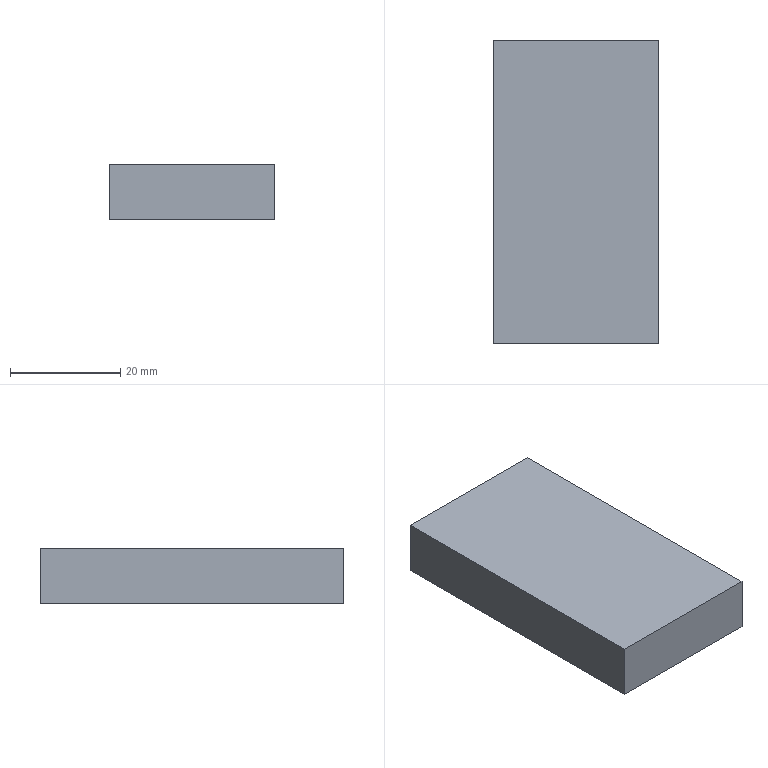Part | NX | features solid 2 | 1 solid | 6 faces | box 30 x 55 x 10 mm | volume 16500 mm3 | plane 6
STEP:
#1=CARTESIAN_POINT('',(660.,90.,-75.));
#2=VERTEX_POINT('',#1);
#3=CARTESIAN_POINT('',(660.,145.,-75.));
#4=VERTEX_POINT('',#3);
#5=CARTESIAN_POINT('',(660.,225.,-75.));
#6=DIRECTION('',(0.,-1.,0.));
#7=VECTOR('',#6,1000.);
#8=LINE('',#5,#7);
#9=EDGE_CURVE('',#2,#4,#8,.F.);
#10=ORIENTED_EDGE('',*,*,#9,.T.);
#11=CARTESIAN_POINT('',(660.,145.,-65.));
#12=VERTEX_POINT('',#11);
#13=CARTESIAN_POINT('',(660.,145.,-75.));
#14=DIRECTION('',(0.,0.,1.));
#15=VECTOR('',#14,1000.);
#16=LINE('',#13,#15);
#17=EDGE_CURVE('',#4,#12,#16,.T.);
#18=ORIENTED_EDGE('',*,*,#17,.T.);
#19=CARTESIAN_POINT('',(660.,90.,-65.));
#20=VERTEX_POINT('',#19);
#21=CARTESIAN_POINT('',(660.,225.,-65.));
#22=DIRECTION('',(0.,1.,0.));
#23=VECTOR('',#22,1000.);
#24=LINE('',#21,#23);
#25=EDGE_CURVE('',#20,#12,#24,.T.);
#26=ORIENTED_EDGE('',*,*,#25,.F.);
#27=CARTESIAN_POINT('',(660.,90.,-75.));
#28=DIRECTION('',(0.,0.,-1.));
#29=VECTOR('',#28,1000.);
#30=LINE('',#27,#29);
#31=EDGE_CURVE('',#20,#2,#30,.T.);
#32=ORIENTED_EDGE('',*,*,#31,.T.);
#33=EDGE_LOOP('',(#10,#18,#26,#32));
#34=FACE_BOUND('',#33,.T.);
#35=CARTESIAN_POINT('',(660.,225.,-75.));
#36=DIRECTION('',(1.,0.,0.));
#37=DIRECTION('',(0.,0.,-1.));
#38=AXIS2_PLACEMENT_3D('',#35,#36,#37);
#39=PLANE('',#38);
#40=ADVANCED_FACE('',(#34),#39,.T.);
#41=CARTESIAN_POINT('',(630.,145.,-65.));
#42=VERTEX_POINT('',#41);
#43=CARTESIAN_POINT('',(585.,145.,-65.));
#44=DIRECTION('',(1.,0.,0.));
#45=VECTOR('',#44,1000.);
#46=LINE('',#43,#45);
#47=EDGE_CURVE('',#42,#12,#46,.T.);
#48=ORIENTED_EDGE('',*,*,#47,.F.);
#49=CARTESIAN_POINT('',(630.,90.,-65.));
#50=VERTEX_POINT('',#49);
#51=CARTESIAN_POINT('',(630.,225.,-65.));
#52=DIRECTION('',(0.,1.,0.));
#53=VECTOR('',#52,1000.);
#54=LINE('',#51,#53);
#55=EDGE_CURVE('',#50,#42,#54,.T.);
#56=ORIENTED_EDGE('',*,*,#55,.F.);
#57=CARTESIAN_POINT('',(585.,90.,-65.));
#58=DIRECTION('',(1.,0.,0.));
#59=VECTOR('',#58,1000.);
#60=LINE('',#57,#59);
#61=EDGE_CURVE('',#50,#20,#60,.T.);
#62=ORIENTED_EDGE('',*,*,#61,.T.);
#63=ORIENTED_EDGE('',*,*,#25,.T.);
#64=EDGE_LOOP('',(#48,#56,#62,#63));
#65=FACE_BOUND('',#64,.T.);
#66=CARTESIAN_POINT('',(585.,225.,-65.));
#67=DIRECTION('',(0.,0.,-1.));
#68=DIRECTION('',(0.,1.,0.));
#69=AXIS2_PLACEMENT_3D('',#66,#67,#68);
#70=PLANE('',#69);
#71=ADVANCED_FACE('',(#65),#70,.F.);
#72=CARTESIAN_POINT('',(630.,145.,-75.));
#73=VERTEX_POINT('',#72);
#74=CARTESIAN_POINT('',(585.,145.,-75.));
#75=DIRECTION('',(1.,0.,0.));
#76=VECTOR('',#75,1000.);
#77=LINE('',#74,#76);
#78=EDGE_CURVE('',#4,#73,#77,.F.);
#79=ORIENTED_EDGE('',*,*,#78,.F.);
#80=ORIENTED_EDGE('',*,*,#9,.F.);
#81=CARTESIAN_POINT('',(630.,90.,-75.));
#82=VERTEX_POINT('',#81);
#83=CARTESIAN_POINT('',(585.,90.,-75.));
#84=DIRECTION('',(1.,0.,0.));
#85=VECTOR('',#84,1000.);
#86=LINE('',#83,#85);
#87=EDGE_CURVE('',#2,#82,#86,.F.);
#88=ORIENTED_EDGE('',*,*,#87,.T.);
#89=CARTESIAN_POINT('',(630.,225.,-75.));
#90=DIRECTION('',(0.,-1.,0.));
#91=VECTOR('',#90,1000.);
#92=LINE('',#89,#91);
#93=EDGE_CURVE('',#82,#73,#92,.F.);
#94=ORIENTED_EDGE('',*,*,#93,.T.);
#95=EDGE_LOOP('',(#79,#80,#88,#94));
#96=FACE_BOUND('',#95,.T.);
#97=CARTESIAN_POINT('',(585.,225.,-75.));
#98=DIRECTION('',(0.,0.,-1.));
#99=DIRECTION('',(0.,1.,0.));
#100=AXIS2_PLACEMENT_3D('',#97,#98,#99);
#101=PLANE('',#100);
#102=ADVANCED_FACE('',(#96),#101,.T.);
#103=ORIENTED_EDGE('',*,*,#93,.F.);
#104=CARTESIAN_POINT('',(630.,90.,-75.));
#105=DIRECTION('',(0.,0.,1.));
#106=VECTOR('',#105,1000.);
#107=LINE('',#104,#106);
#108=EDGE_CURVE('',#82,#50,#107,.T.);
#109=ORIENTED_EDGE('',*,*,#108,.T.);
#110=ORIENTED_EDGE('',*,*,#55,.T.);
#111=CARTESIAN_POINT('',(630.,145.,-75.));
#112=DIRECTION('',(0.,0.,1.));
#113=VECTOR('',#112,1000.);
#114=LINE('',#111,#113);
#115=EDGE_CURVE('',#42,#73,#114,.F.);
#116=ORIENTED_EDGE('',*,*,#115,.T.);
#117=EDGE_LOOP('',(#103,#109,#110,#116));
#118=FACE_BOUND('',#117,.T.);
#119=CARTESIAN_POINT('',(630.,225.,-75.));
#120=DIRECTION('',(1.,0.,0.));
#121=DIRECTION('',(0.,0.,-1.));
#122=AXIS2_PLACEMENT_3D('',#119,#120,#121);
#123=PLANE('',#122);
#124=ADVANCED_FACE('',(#118),#123,.F.);
#125=ORIENTED_EDGE('',*,*,#108,.F.);
#126=ORIENTED_EDGE('',*,*,#87,.F.);
#127=ORIENTED_EDGE('',*,*,#31,.F.);
#128=ORIENTED_EDGE('',*,*,#61,.F.);
#129=EDGE_LOOP('',(#125,#126,#127,#128));
#130=FACE_BOUND('',#129,.T.);
#131=CARTESIAN_POINT('',(670.,90.,-10.));
#132=DIRECTION('',(0.,1.,0.));
#133=DIRECTION('',(0.,0.,1.));
#134=AXIS2_PLACEMENT_3D('',#131,#132,#133);
#135=PLANE('',#134);
#136=ADVANCED_FACE('',(#130),#135,.F.);
#137=ORIENTED_EDGE('',*,*,#115,.F.);
#138=ORIENTED_EDGE('',*,*,#47,.T.);
#139=ORIENTED_EDGE('',*,*,#17,.F.);
#140=ORIENTED_EDGE('',*,*,#78,.T.);
#141=EDGE_LOOP('',(#137,#138,#139,#140));
#142=FACE_BOUND('',#141,.T.);
#143=CARTESIAN_POINT('',(585.,145.,-75.));
#144=DIRECTION('',(0.,1.,0.));
#145=DIRECTION('',(0.,0.,1.));
#146=AXIS2_PLACEMENT_3D('',#143,#144,#145);
#147=PLANE('',#146);
#148=ADVANCED_FACE('',(#142),#147,.T.);
#149=CLOSED_SHELL('',(#40,#71,#102,#124,#136,#148));
#150=MANIFOLD_SOLID_BREP('',#149);
#151=(LENGTH_UNIT()NAMED_UNIT(*)SI_UNIT(.MILLI.,.METRE.));
#152=UNCERTAINTY_MEASURE_WITH_UNIT(LENGTH_MEASURE(0.00001),#151,'','');
#153=(NAMED_UNIT(*)PLANE_ANGLE_UNIT()SI_UNIT($,.RADIAN.));
#154=(NAMED_UNIT(*)SI_UNIT($,.STERADIAN.)SOLID_ANGLE_UNIT());
#155=(GEOMETRIC_REPRESENTATION_CONTEXT(3)GLOBAL_UNCERTAINTY_ASSIGNED_CONTEXT((#152))GLOBAL_UNIT_ASSIGNED_CONTEXT((#151,#153,#154))REPRESENTATION_CONTEXT('',''));
#156=ADVANCED_BREP_SHAPE_REPRESENTATION('',(#150),#155);